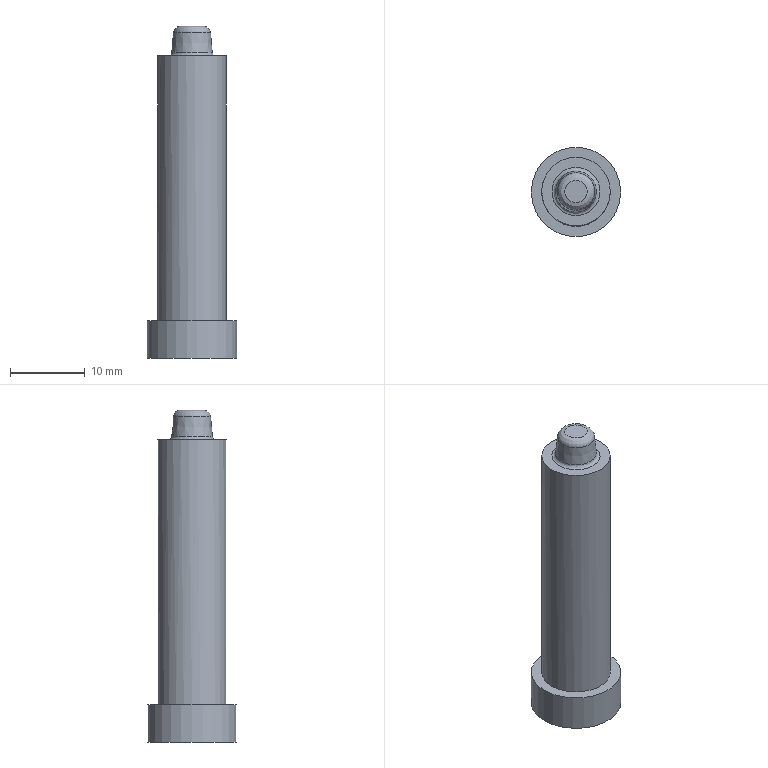Part | NX | features solid 2 | 1 solid | 9 faces | box 12 x 12 x 44.5 mm | volume 3009 mm3 | plane 4 | cylinder 2 | torus 2 | cone 1 | commonest cylinder face diameters 9.2 x1 12 x1
STEP:
#1=CARTESIAN_POINT('',(3399.266,-906.707,823.716));
#2=VERTEX_POINT('',#1);
#3=CARTESIAN_POINT('',(3405.266,-906.707,823.716));
#4=DIRECTION('',(0.,0.,-1.));
#5=DIRECTION('',(-1.,0.,0.));
#6=AXIS2_PLACEMENT_3D('',#3,#4,#5);
#7=CIRCLE('',#6,6.);
#8=EDGE_CURVE('',#2,#2,#7,.F.);
#9=ORIENTED_EDGE('',*,*,#8,.T.);
#10=EDGE_LOOP('',(#9));
#11=FACE_BOUND('',#10,.T.);
#12=CARTESIAN_POINT('',(3399.266,-906.707,828.716));
#13=VERTEX_POINT('',#12);
#14=CARTESIAN_POINT('',(3405.266,-906.707,828.716));
#15=DIRECTION('',(0.,0.,-1.));
#16=DIRECTION('',(-1.,0.,0.));
#17=AXIS2_PLACEMENT_3D('',#14,#15,#16);
#18=CIRCLE('',#17,6.);
#19=EDGE_CURVE('',#13,#13,#18,.F.);
#20=ORIENTED_EDGE('',*,*,#19,.F.);
#21=EDGE_LOOP('',(#20));
#22=FACE_BOUND('',#21,.T.);
#23=CARTESIAN_POINT('',(3405.266,-906.707,823.716));
#24=DIRECTION('',(0.,0.,1.));
#25=DIRECTION('',(1.,0.,0.));
#26=AXIS2_PLACEMENT_3D('',#23,#24,#25);
#27=CYLINDRICAL_SURFACE('',#26,6.);
#28=ADVANCED_FACE('',(#11,#22),#27,.T.);
#29=ORIENTED_EDGE('',*,*,#8,.F.);
#30=EDGE_LOOP('',(#29));
#31=FACE_BOUND('',#30,.T.);
#32=CARTESIAN_POINT('',(3405.266,-906.707,823.716));
#33=DIRECTION('',(0.,0.,-1.));
#34=DIRECTION('',(-1.,0.,0.));
#35=AXIS2_PLACEMENT_3D('',#32,#33,#34);
#36=PLANE('',#35);
#37=ADVANCED_FACE('',(#31),#36,.T.);
#38=CARTESIAN_POINT('',(3409.866,-906.707,828.716));
#39=VERTEX_POINT('',#38);
#40=CARTESIAN_POINT('',(3405.266,-906.707,828.716));
#41=DIRECTION('',(0.,0.,1.));
#42=DIRECTION('',(1.,0.,0.));
#43=AXIS2_PLACEMENT_3D('',#40,#41,#42);
#44=CIRCLE('',#43,4.6);
#45=EDGE_CURVE('',#39,#39,#44,.T.);
#46=ORIENTED_EDGE('',*,*,#45,.F.);
#47=EDGE_LOOP('',(#46));
#48=FACE_BOUND('',#47,.T.);
#49=ORIENTED_EDGE('',*,*,#19,.T.);
#50=EDGE_LOOP('',(#49));
#51=FACE_BOUND('',#50,.T.);
#52=CARTESIAN_POINT('',(3405.266,-906.707,828.716));
#53=DIRECTION('',(0.,0.,-1.));
#54=DIRECTION('',(-1.,0.,0.));
#55=AXIS2_PLACEMENT_3D('',#52,#53,#54);
#56=PLANE('',#55);
#57=ADVANCED_FACE('',(#48,#51),#56,.F.);
#58=CARTESIAN_POINT('',(3405.266,-903.473,864.216));
#59=VERTEX_POINT('',#58);
#60=CARTESIAN_POINT('',(3405.266,-906.707,864.216));
#61=DIRECTION('',(0.,0.,-1.));
#62=DIRECTION('',(0.,1.,0.));
#63=AXIS2_PLACEMENT_3D('',#60,#61,#62);
#64=CIRCLE('',#63,3.233);
#65=EDGE_CURVE('',#59,#59,#64,.T.);
#66=ORIENTED_EDGE('',*,*,#65,.T.);
#67=EDGE_LOOP('',(#66));
#68=FACE_BOUND('',#67,.T.);
#69=CARTESIAN_POINT('',(3405.266,-902.107,864.216));
#70=VERTEX_POINT('',#69);
#71=CARTESIAN_POINT('',(3405.266,-906.707,864.216));
#72=DIRECTION('',(0.,0.,-1.));
#73=DIRECTION('',(0.,1.,0.));
#74=AXIS2_PLACEMENT_3D('',#71,#72,#73);
#75=CIRCLE('',#74,4.6);
#76=EDGE_CURVE('',#70,#70,#75,.T.);
#77=ORIENTED_EDGE('',*,*,#76,.F.);
#78=EDGE_LOOP('',(#77));
#79=FACE_BOUND('',#78,.T.);
#80=CARTESIAN_POINT('',(3426.074,-912.553,864.216));
#81=DIRECTION('',(0.,0.,-1.));
#82=DIRECTION('',(0.,1.,0.));
#83=AXIS2_PLACEMENT_3D('',#80,#81,#82);
#84=PLANE('',#83);
#85=ADVANCED_FACE('',(#68,#79),#84,.F.);
#86=ORIENTED_EDGE('',*,*,#76,.T.);
#87=EDGE_LOOP('',(#86));
#88=FACE_BOUND('',#87,.T.);
#89=ORIENTED_EDGE('',*,*,#45,.T.);
#90=EDGE_LOOP('',(#89));
#91=FACE_BOUND('',#90,.T.);
#92=CARTESIAN_POINT('',(3405.266,-906.707,823.716));
#93=DIRECTION('',(0.,0.,1.));
#94=DIRECTION('',(1.,0.,0.));
#95=AXIS2_PLACEMENT_3D('',#92,#93,#94);
#96=CYLINDRICAL_SURFACE('',#95,4.6);
#97=ADVANCED_FACE('',(#88,#91),#96,.T.);
#98=CARTESIAN_POINT('',(3405.266,-909.212,867.303));
#99=VERTEX_POINT('',#98);
#100=CARTESIAN_POINT('',(3405.266,-906.707,867.303));
#101=DIRECTION('',(0.,0.,1.));
#102=DIRECTION('',(0.,-1.,0.));
#103=AXIS2_PLACEMENT_3D('',#100,#101,#102);
#104=CIRCLE('',#103,2.505);
#105=EDGE_CURVE('',#99,#99,#104,.F.);
#106=ORIENTED_EDGE('',*,*,#105,.T.);
#107=EDGE_LOOP('',(#106));
#108=FACE_BOUND('',#107,.T.);
#109=CARTESIAN_POINT('',(3405.266,-903.972,864.673));
#110=VERTEX_POINT('',#109);
#111=CARTESIAN_POINT('',(3405.266,-906.707,864.673));
#112=DIRECTION('',(0.,0.,-1.));
#113=DIRECTION('',(0.,1.,0.));
#114=AXIS2_PLACEMENT_3D('',#111,#112,#113);
#115=CIRCLE('',#114,2.735);
#116=EDGE_CURVE('',#110,#110,#115,.F.);
#117=ORIENTED_EDGE('',*,*,#116,.T.);
#118=EDGE_LOOP('',(#117));
#119=FACE_BOUND('',#118,.T.);
#120=CARTESIAN_POINT('',(3405.266,-906.707,864.216));
#121=DIRECTION('',(0.,0.,-1.));
#122=DIRECTION('',(0.,-1.,0.));
#123=AXIS2_PLACEMENT_3D('',#120,#121,#122);
#124=CONICAL_SURFACE('',#123,2.775,0.08727);
#125=ADVANCED_FACE('',(#108,#119),#124,.T.);
#126=CARTESIAN_POINT('',(3405.266,-905.198,868.216));
#127=VERTEX_POINT('',#126);
#128=CARTESIAN_POINT('',(3405.266,-906.707,868.216));
#129=DIRECTION('',(0.,0.,-1.));
#130=DIRECTION('',(0.,1.,0.));
#131=AXIS2_PLACEMENT_3D('',#128,#129,#130);
#132=CIRCLE('',#131,1.509);
#133=EDGE_CURVE('',#127,#127,#132,.F.);
#134=ORIENTED_EDGE('',*,*,#133,.T.);
#135=EDGE_LOOP('',(#134));
#136=FACE_BOUND('',#135,.T.);
#137=CARTESIAN_POINT('',(3426.074,-912.553,868.216));
#138=DIRECTION('',(0.,0.,-1.));
#139=DIRECTION('',(0.,1.,0.));
#140=AXIS2_PLACEMENT_3D('',#137,#138,#139);
#141=PLANE('',#140);
#142=ADVANCED_FACE('',(#136),#141,.F.);
#143=ORIENTED_EDGE('',*,*,#116,.F.);
#144=EDGE_LOOP('',(#143));
#145=FACE_BOUND('',#144,.T.);
#146=ORIENTED_EDGE('',*,*,#65,.F.);
#147=EDGE_LOOP('',(#146));
#148=FACE_BOUND('',#147,.T.);
#149=CARTESIAN_POINT('',(3405.266,-906.707,864.716));
#150=DIRECTION('',(0.,0.,-1.));
#151=DIRECTION('',(0.,1.,0.));
#152=AXIS2_PLACEMENT_3D('',#149,#150,#151);
#153=TOROIDAL_SURFACE('',#152,3.233,0.5);
#154=ADVANCED_FACE('',(#145,#148),#153,.F.);
#155=ORIENTED_EDGE('',*,*,#133,.F.);
#156=EDGE_LOOP('',(#155));
#157=FACE_BOUND('',#156,.T.);
#158=ORIENTED_EDGE('',*,*,#105,.F.);
#159=EDGE_LOOP('',(#158));
#160=FACE_BOUND('',#159,.T.);
#161=CARTESIAN_POINT('',(3405.266,-906.707,867.216));
#162=DIRECTION('',(0.,0.,-1.));
#163=DIRECTION('',(0.,1.,0.));
#164=AXIS2_PLACEMENT_3D('',#161,#162,#163);
#165=TOROIDAL_SURFACE('',#164,1.509,1.);
#166=ADVANCED_FACE('',(#157,#160),#165,.T.);
#167=CLOSED_SHELL('',(#28,#37,#57,#85,#97,#125,#142,#154,#166));
#168=MANIFOLD_SOLID_BREP('',#167);
#169=(LENGTH_UNIT()NAMED_UNIT(*)SI_UNIT(.MILLI.,.METRE.));
#170=UNCERTAINTY_MEASURE_WITH_UNIT(LENGTH_MEASURE(0.00001),#169,'','');
#171=(NAMED_UNIT(*)PLANE_ANGLE_UNIT()SI_UNIT($,.RADIAN.));
#172=(NAMED_UNIT(*)SI_UNIT($,.STERADIAN.)SOLID_ANGLE_UNIT());
#173=(GEOMETRIC_REPRESENTATION_CONTEXT(3)GLOBAL_UNCERTAINTY_ASSIGNED_CONTEXT((#170))GLOBAL_UNIT_ASSIGNED_CONTEXT((#169,#171,#172))REPRESENTATION_CONTEXT('',''));
#174=ADVANCED_BREP_SHAPE_REPRESENTATION('',(#168),#173);